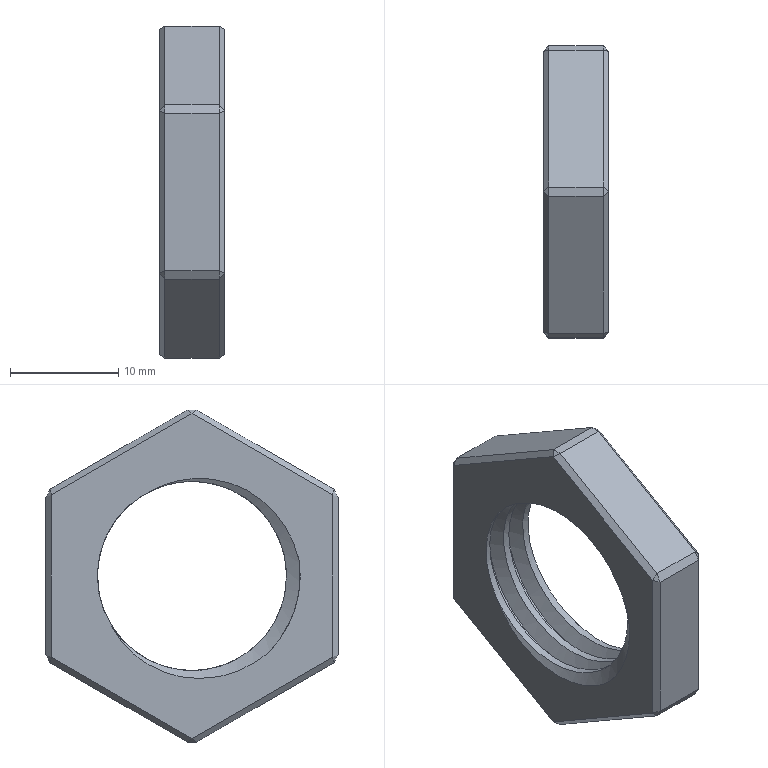Part | STEP file | Tube feed_id834_x_t | 1 solid | 43 faces | box 6 x 27 x 30.677 mm | volume 2131 mm3 | plane 39 | spline 2 | cylinder 2 | commonest cylinder face diameters 17.5 x1 20 x1